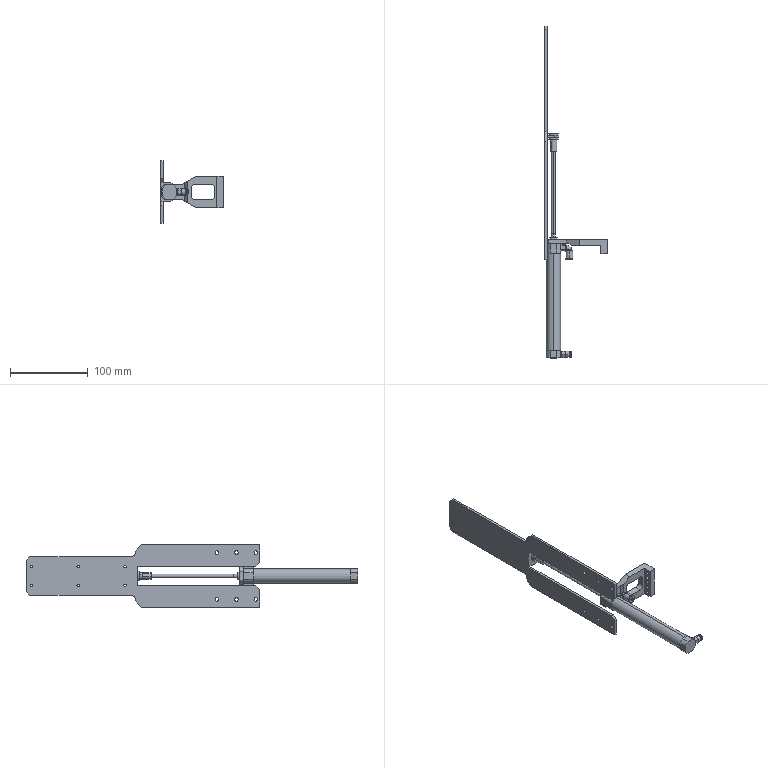Part | SolidWorks | 6 solids | 266 faces | box 80 x 426 x 80 mm | volume 107986 mm3 | plane 120 | cylinder 108 | cone 36 | spline 2 | commonest cylinder face diameters 4.5 x18 3.3 x12 10 x10 4.2 x8 5 x8 20 x8